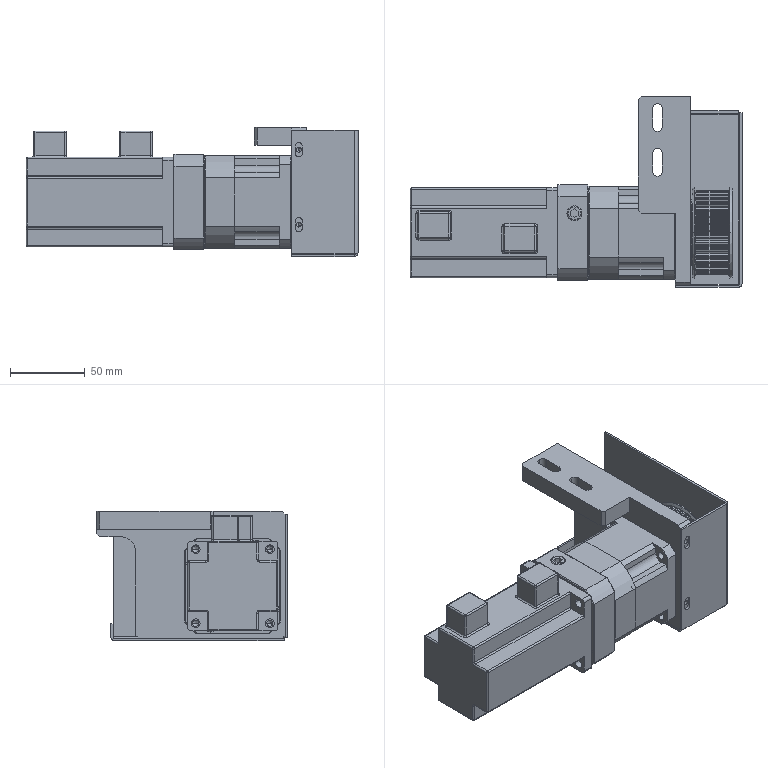Part | SolidWorks | 24 solids | 1253 faces | box 221.9 x 127.5 x 86.5 mm | volume 738025 mm3 | cylinder 562 | plane 463 | cone 162 | torus 37 | sphere 16 | spline 13 | commonest cylinder face diameters 0.8 x91 1.2 x90 2 x51 52.85 x39 56.45 x36 4.2 x28